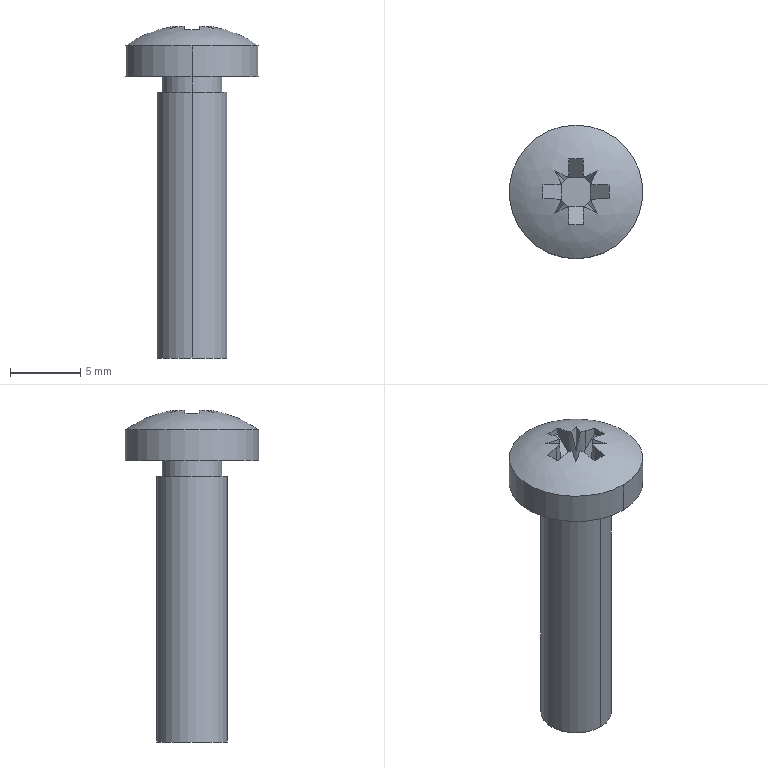Part | SolidWorks | features BaseBody 1 | 1 solid | 51 faces | box 9.5 x 9.5 x 23.612 mm | volume 579.898 mm3 | plane 40 | cylinder 10 | spline 1 | commonest cylinder face diameters 2 x4 4.25 x2 5 x2 9.5 x2